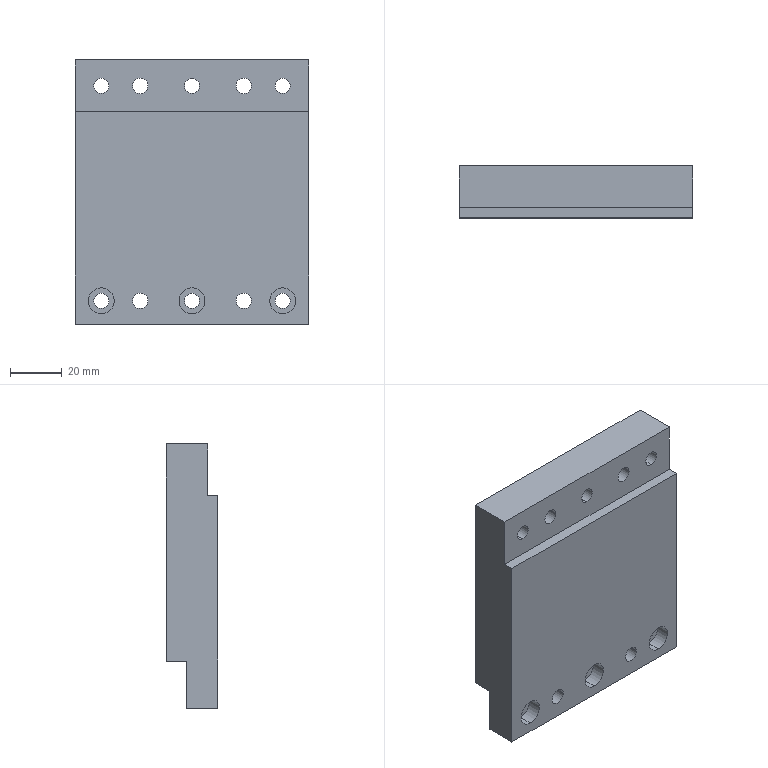Part | NX | features BREP 1 | 1 solid | 48 faces | box 90 x 20 x 102 mm | volume 157949 mm3 | cylinder 32 | plane 16 | commonest cylinder face diameters 5.8 x12 10 x12 6 x8
STEP:
#1=CARTESIAN_POINT('',(35.,20.,36.));
#2=VERTEX_POINT('',#1);
#3=CARTESIAN_POINT('',(35.,14.6,36.));
#4=VERTEX_POINT('',#3);
#5=CARTESIAN_POINT('',(35.,20.,36.));
#6=DIRECTION('',(0.,-1.,0.));
#7=VECTOR('',#6,1000.);
#8=LINE('',#5,#7);
#9=EDGE_CURVE('',#2,#4,#8,.T.);
#10=ORIENTED_EDGE('',*,*,#9,.F.);
#11=CARTESIAN_POINT('',(35.,20.,46.));
#12=VERTEX_POINT('',#11);
#13=CARTESIAN_POINT('',(35.,20.,41.));
#14=DIRECTION('',(0.,-1.,0.));
#15=DIRECTION('',(0.,0.,1.));
#16=AXIS2_PLACEMENT_3D('',#13,#14,#15);
#17=CIRCLE('',#16,5.);
#18=EDGE_CURVE('',#12,#2,#17,.T.);
#19=ORIENTED_EDGE('',*,*,#18,.F.);
#20=CARTESIAN_POINT('',(35.,14.6,46.));
#21=VERTEX_POINT('',#20);
#22=CARTESIAN_POINT('',(35.,20.,46.));
#23=DIRECTION('',(0.,-1.,0.));
#24=VECTOR('',#23,1000.);
#25=LINE('',#22,#24);
#26=EDGE_CURVE('',#12,#21,#25,.T.);
#27=ORIENTED_EDGE('',*,*,#26,.T.);
#28=CARTESIAN_POINT('',(35.,14.6,41.));
#29=DIRECTION('',(0.,1.,0.));
#30=DIRECTION('',(0.,0.,-1.));
#31=AXIS2_PLACEMENT_3D('',#28,#29,#30);
#32=CIRCLE('',#31,5.);
#33=EDGE_CURVE('',#4,#21,#32,.T.);
#34=ORIENTED_EDGE('',*,*,#33,.F.);
#35=EDGE_LOOP('',(#10,#19,#27,#34));
#36=FACE_BOUND('',#35,.T.);
#37=CARTESIAN_POINT('',(35.,20.,41.));
#38=DIRECTION('',(0.,1.,0.));
#39=DIRECTION('',(0.,0.,1.));
#40=AXIS2_PLACEMENT_3D('',#37,#38,#39);
#41=CYLINDRICAL_SURFACE('',#40,5.);
#42=ADVANCED_FACE('',(#36),#41,.F.);
#43=ORIENTED_EDGE('',*,*,#33,.T.);
#44=CARTESIAN_POINT('',(35.,14.6,41.));
#45=DIRECTION('',(0.,1.,0.));
#46=DIRECTION('',(0.,0.,1.));
#47=AXIS2_PLACEMENT_3D('',#44,#45,#46);
#48=CIRCLE('',#47,5.);
#49=EDGE_CURVE('',#21,#4,#48,.T.);
#50=ORIENTED_EDGE('',*,*,#49,.T.);
#51=EDGE_LOOP('',(#43,#50));
#52=FACE_BOUND('',#51,.T.);
#53=CARTESIAN_POINT('',(35.,14.6,43.9));
#54=VERTEX_POINT('',#53);
#55=CARTESIAN_POINT('',(35.,14.6,38.1));
#56=VERTEX_POINT('',#55);
#57=CARTESIAN_POINT('',(35.,14.6,41.));
#58=DIRECTION('',(0.,-1.,0.));
#59=DIRECTION('',(0.,0.,1.));
#60=AXIS2_PLACEMENT_3D('',#57,#58,#59);
#61=CIRCLE('',#60,2.9);
#62=EDGE_CURVE('',#54,#56,#61,.T.);
#63=ORIENTED_EDGE('',*,*,#62,.T.);
#64=CARTESIAN_POINT('',(35.,14.6,41.));
#65=DIRECTION('',(0.,-1.,0.));
#66=DIRECTION('',(0.,0.,-1.));
#67=AXIS2_PLACEMENT_3D('',#64,#65,#66);
#68=CIRCLE('',#67,2.9);
#69=EDGE_CURVE('',#56,#54,#68,.T.);
#70=ORIENTED_EDGE('',*,*,#69,.T.);
#71=EDGE_LOOP('',(#63,#70));
#72=FACE_BOUND('',#71,.T.);
#73=CARTESIAN_POINT('',(37.9,14.6,41.));
#74=DIRECTION('',(0.,-1.,0.));
#75=DIRECTION('',(0.,0.,-1.));
#76=AXIS2_PLACEMENT_3D('',#73,#74,#75);
#77=PLANE('',#76);
#78=ADVANCED_FACE('',(#52,#72),#77,.F.);
#79=ORIENTED_EDGE('',*,*,#49,.F.);
#80=ORIENTED_EDGE('',*,*,#26,.F.);
#81=CARTESIAN_POINT('',(35.,20.,41.));
#82=DIRECTION('',(0.,-1.,0.));
#83=DIRECTION('',(0.,0.,-1.));
#84=AXIS2_PLACEMENT_3D('',#81,#82,#83);
#85=CIRCLE('',#84,5.);
#86=EDGE_CURVE('',#2,#12,#85,.T.);
#87=ORIENTED_EDGE('',*,*,#86,.F.);
#88=ORIENTED_EDGE('',*,*,#9,.T.);
#89=EDGE_LOOP('',(#79,#80,#87,#88));
#90=FACE_BOUND('',#89,.T.);
#91=CARTESIAN_POINT('',(35.,20.,41.));
#92=DIRECTION('',(0.,1.,0.));
#93=DIRECTION('',(0.,0.,1.));
#94=AXIS2_PLACEMENT_3D('',#91,#92,#93);
#95=CYLINDRICAL_SURFACE('',#94,5.);
#96=ADVANCED_FACE('',(#90),#95,.F.);
#97=CARTESIAN_POINT('',(-45.,20.,51.));
#98=VERTEX_POINT('',#97);
#99=CARTESIAN_POINT('',(-45.,20.,-33.));
#100=VERTEX_POINT('',#99);
#101=CARTESIAN_POINT('',(-45.,20.,51.));
#102=DIRECTION('',(0.,0.,-1.));
#103=VECTOR('',#102,1000.);
#104=LINE('',#101,#103);
#105=EDGE_CURVE('',#98,#100,#104,.T.);
#106=ORIENTED_EDGE('',*,*,#105,.F.);
#107=CARTESIAN_POINT('',(45.,20.,51.));
#108=VERTEX_POINT('',#107);
#109=CARTESIAN_POINT('',(45.,20.,51.));
#110=DIRECTION('',(-1.,0.,0.));
#111=VECTOR('',#110,1000.);
#112=LINE('',#109,#111);
#113=EDGE_CURVE('',#108,#98,#112,.T.);
#114=ORIENTED_EDGE('',*,*,#113,.F.);
#115=CARTESIAN_POINT('',(45.,20.,-33.));
#116=VERTEX_POINT('',#115);
#117=CARTESIAN_POINT('',(45.,20.,-33.));
#118=DIRECTION('',(0.,0.,1.));
#119=VECTOR('',#118,1000.);
#120=LINE('',#117,#119);
#121=EDGE_CURVE('',#116,#108,#120,.T.);
#122=ORIENTED_EDGE('',*,*,#121,.F.);
#123=CARTESIAN_POINT('',(45.,20.,-33.));
#124=DIRECTION('',(-1.,0.,0.));
#125=VECTOR('',#124,1000.);
#126=LINE('',#123,#125);
#127=EDGE_CURVE('',#116,#100,#126,.T.);
#128=ORIENTED_EDGE('',*,*,#127,.T.);
#129=EDGE_LOOP('',(#106,#114,#122,#128));
#130=FACE_BOUND('',#129,.T.);
#131=ORIENTED_EDGE('',*,*,#18,.T.);
#132=ORIENTED_EDGE('',*,*,#86,.T.);
#133=EDGE_LOOP('',(#131,#132));
#134=FACE_BOUND('',#133,.T.);
#135=CARTESIAN_POINT('',(0.,20.,46.));
#136=VERTEX_POINT('',#135);
#137=CARTESIAN_POINT('',(0.,20.,36.));
#138=VERTEX_POINT('',#137);
#139=CARTESIAN_POINT('',(0.,20.,41.));
#140=DIRECTION('',(0.,-1.,0.));
#141=DIRECTION('',(0.,0.,1.));
#142=AXIS2_PLACEMENT_3D('',#139,#140,#141);
#143=CIRCLE('',#142,5.);
#144=EDGE_CURVE('',#136,#138,#143,.T.);
#145=ORIENTED_EDGE('',*,*,#144,.T.);
#146=CARTESIAN_POINT('',(0.,20.,41.));
#147=DIRECTION('',(0.,-1.,0.));
#148=DIRECTION('',(0.,0.,-1.));
#149=AXIS2_PLACEMENT_3D('',#146,#147,#148);
#150=CIRCLE('',#149,5.);
#151=EDGE_CURVE('',#138,#136,#150,.T.);
#152=ORIENTED_EDGE('',*,*,#151,.T.);
#153=EDGE_LOOP('',(#145,#152));
#154=FACE_BOUND('',#153,.T.);
#155=CARTESIAN_POINT('',(-35.,20.,46.));
#156=VERTEX_POINT('',#155);
#157=CARTESIAN_POINT('',(-35.,20.,36.));
#158=VERTEX_POINT('',#157);
#159=CARTESIAN_POINT('',(-35.,20.,41.));
#160=DIRECTION('',(0.,-1.,0.));
#161=DIRECTION('',(0.,0.,1.));
#162=AXIS2_PLACEMENT_3D('',#159,#160,#161);
#163=CIRCLE('',#162,5.);
#164=EDGE_CURVE('',#156,#158,#163,.T.);
#165=ORIENTED_EDGE('',*,*,#164,.T.);
#166=CARTESIAN_POINT('',(-35.,20.,41.));
#167=DIRECTION('',(0.,-1.,0.));
#168=DIRECTION('',(0.,0.,-1.));
#169=AXIS2_PLACEMENT_3D('',#166,#167,#168);
#170=CIRCLE('',#169,5.);
#171=EDGE_CURVE('',#158,#156,#170,.T.);
#172=ORIENTED_EDGE('',*,*,#171,.T.);
#173=EDGE_LOOP('',(#165,#172));
#174=FACE_BOUND('',#173,.T.);
#175=CARTESIAN_POINT('',(17.,20.,41.));
#176=VERTEX_POINT('',#175);
#177=CARTESIAN_POINT('',(23.,20.,41.));
#178=VERTEX_POINT('',#177);
#179=CARTESIAN_POINT('',(20.,20.,41.));
#180=DIRECTION('',(0.,-1.,0.));
#181=DIRECTION('',(-1.,0.,0.));
#182=AXIS2_PLACEMENT_3D('',#179,#180,#181);
#183=CIRCLE('',#182,3.);
#184=EDGE_CURVE('',#176,#178,#183,.T.);
#185=ORIENTED_EDGE('',*,*,#184,.T.);
#186=CARTESIAN_POINT('',(20.,20.,41.));
#187=DIRECTION('',(0.,-1.,0.));
#188=DIRECTION('',(1.,0.,0.));
#189=AXIS2_PLACEMENT_3D('',#186,#187,#188);
#190=CIRCLE('',#189,3.);
#191=EDGE_CURVE('',#178,#176,#190,.T.);
#192=ORIENTED_EDGE('',*,*,#191,.T.);
#193=EDGE_LOOP('',(#185,#192));
#194=FACE_BOUND('',#193,.T.);
#195=CARTESIAN_POINT('',(-23.,20.,41.));
#196=VERTEX_POINT('',#195);
#197=CARTESIAN_POINT('',(-17.,20.,41.));
#198=VERTEX_POINT('',#197);
#199=CARTESIAN_POINT('',(-20.,20.,41.));
#200=DIRECTION('',(0.,-1.,0.));
#201=DIRECTION('',(-1.,0.,0.));
#202=AXIS2_PLACEMENT_3D('',#199,#200,#201);
#203=CIRCLE('',#202,3.);
#204=EDGE_CURVE('',#196,#198,#203,.T.);
#205=ORIENTED_EDGE('',*,*,#204,.T.);
#206=CARTESIAN_POINT('',(-20.,20.,41.));
#207=DIRECTION('',(0.,-1.,0.));
#208=DIRECTION('',(1.,0.,0.));
#209=AXIS2_PLACEMENT_3D('',#206,#207,#208);
#210=CIRCLE('',#209,3.);
#211=EDGE_CURVE('',#198,#196,#210,.T.);
#212=ORIENTED_EDGE('',*,*,#211,.T.);
#213=EDGE_LOOP('',(#205,#212));
#214=FACE_BOUND('',#213,.T.);
#215=CARTESIAN_POINT('',(-45.,20.,51.));
#216=DIRECTION('',(0.,1.,0.));
#217=DIRECTION('',(1.,0.,0.));
#218=AXIS2_PLACEMENT_3D('',#215,#216,#217);
#219=PLANE('',#218);
#220=ADVANCED_FACE('',(#130,#134,#154,#174,#194,#214),#219,.T.);
#221=CARTESIAN_POINT('',(45.,12.,-33.));
#222=VERTEX_POINT('',#221);
#223=CARTESIAN_POINT('',(-45.,12.,-33.));
#224=VERTEX_POINT('',#223);
#225=CARTESIAN_POINT('',(45.,12.,-33.));
#226=DIRECTION('',(-1.,0.,0.));
#227=VECTOR('',#226,1000.);
#228=LINE('',#225,#227);
#229=EDGE_CURVE('',#222,#224,#228,.T.);
#230=ORIENTED_EDGE('',*,*,#229,.T.);
#231=CARTESIAN_POINT('',(-45.,12.,-33.));
#232=DIRECTION('',(0.,1.,0.));
#233=VECTOR('',#232,1000.);
#234=LINE('',#231,#233);
#235=EDGE_CURVE('',#224,#100,#234,.T.);
#236=ORIENTED_EDGE('',*,*,#235,.T.);
#237=ORIENTED_EDGE('',*,*,#127,.F.);
#238=CARTESIAN_POINT('',(45.,12.,-33.));
#239=DIRECTION('',(0.,1.,0.));
#240=VECTOR('',#239,1000.);
#241=LINE('',#238,#240);
#242=EDGE_CURVE('',#222,#116,#241,.T.);
#243=ORIENTED_EDGE('',*,*,#242,.F.);
#244=EDGE_LOOP('',(#230,#236,#237,#243));
#245=FACE_BOUND('',#244,.T.);
#246=CARTESIAN_POINT('',(-45.,20.,-33.));
#247=DIRECTION('',(0.,0.,1.));
#248=DIRECTION('',(1.,0.,0.));
#249=AXIS2_PLACEMENT_3D('',#246,#247,#248);
#250=PLANE('',#249);
#251=ADVANCED_FACE('',(#245),#250,.F.);
#252=CARTESIAN_POINT('',(45.,0.,31.));
#253=VERTEX_POINT('',#252);
#254=CARTESIAN_POINT('',(45.,4.,31.));
#255=VERTEX_POINT('',#254);
#256=CARTESIAN_POINT('',(45.,0.,31.));
#257=DIRECTION('',(0.,1.,0.));
#258=VECTOR('',#257,1000.);
#259=LINE('',#256,#258);
#260=EDGE_CURVE('',#253,#255,#259,.T.);
#261=ORIENTED_EDGE('',*,*,#260,.F.);
#262=CARTESIAN_POINT('',(45.,0.,-51.));
#263=VERTEX_POINT('',#262);
#264=CARTESIAN_POINT('',(45.,0.,-51.));
#265=DIRECTION('',(0.,0.,1.));
#266=VECTOR('',#265,1000.);
#267=LINE('',#264,#266);
#268=EDGE_CURVE('',#263,#253,#267,.T.);
#269=ORIENTED_EDGE('',*,*,#268,.F.);
#270=CARTESIAN_POINT('',(45.,12.,-51.));
#271=VERTEX_POINT('',#270);
#272=CARTESIAN_POINT('',(45.,0.,-51.));
#273=DIRECTION('',(0.,1.,0.));
#274=VECTOR('',#273,1000.);
#275=LINE('',#272,#274);
#276=EDGE_CURVE('',#263,#271,#275,.T.);
#277=ORIENTED_EDGE('',*,*,#276,.T.);
#278=CARTESIAN_POINT('',(45.,12.,-51.));
#279=DIRECTION('',(0.,0.,1.));
#280=VECTOR('',#279,1000.);
#281=LINE('',#278,#280);
#282=EDGE_CURVE('',#271,#222,#281,.T.);
#283=ORIENTED_EDGE('',*,*,#282,.T.);
#284=ORIENTED_EDGE('',*,*,#242,.T.);
#285=ORIENTED_EDGE('',*,*,#121,.T.);
#286=CARTESIAN_POINT('',(45.,4.,51.));
#287=VERTEX_POINT('',#286);
#288=CARTESIAN_POINT('',(45.,4.,51.));
#289=DIRECTION('',(0.,1.,0.));
#290=VECTOR('',#289,1000.);
#291=LINE('',#288,#290);
#292=EDGE_CURVE('',#287,#108,#291,.T.);
#293=ORIENTED_EDGE('',*,*,#292,.F.);
#294=CARTESIAN_POINT('',(45.,4.,51.));
#295=DIRECTION('',(0.,0.,-1.));
#296=VECTOR('',#295,1000.);
#297=LINE('',#294,#296);
#298=EDGE_CURVE('',#287,#255,#297,.T.);
#299=ORIENTED_EDGE('',*,*,#298,.T.);
#300=EDGE_LOOP('',(#261,#269,#277,#283,#284,#285,#293,#299));
#301=FACE_BOUND('',#300,.T.);
#302=CARTESIAN_POINT('',(45.,20.,-51.));
#303=DIRECTION('',(-1.,0.,0.));
#304=DIRECTION('',(0.,0.,1.));
#305=AXIS2_PLACEMENT_3D('',#302,#303,#304);
#306=PLANE('',#305);
#307=ADVANCED_FACE('',(#301),#306,.F.);
#308=CARTESIAN_POINT('',(-45.,4.,31.));
#309=VERTEX_POINT('',#308);
#310=CARTESIAN_POINT('',(45.,4.,31.));
#311=DIRECTION('',(-1.,0.,0.));
#312=VECTOR('',#311,1000.);
#313=LINE('',#310,#312);
#314=EDGE_CURVE('',#255,#309,#313,.T.);
#315=ORIENTED_EDGE('',*,*,#314,.F.);
#316=ORIENTED_EDGE('',*,*,#298,.F.);
#317=CARTESIAN_POINT('',(-45.,4.,51.));
#318=VERTEX_POINT('',#317);
#319=CARTESIAN_POINT('',(-45.,4.,51.));
#320=DIRECTION('',(1.,0.,0.));
#321=VECTOR('',#320,1000.);
#322=LINE('',#319,#321);
#323=EDGE_CURVE('',#318,#287,#322,.T.);
#324=ORIENTED_EDGE('',*,*,#323,.F.);
#325=CARTESIAN_POINT('',(-45.,4.,31.));
#326=DIRECTION('',(0.,0.,1.));
#327=VECTOR('',#326,1000.);
#328=LINE('',#325,#327);
#329=EDGE_CURVE('',#309,#318,#328,.T.);
#330=ORIENTED_EDGE('',*,*,#329,.F.);
#331=EDGE_LOOP('',(#315,#316,#324,#330));
#332=FACE_BOUND('',#331,.T.);
#333=CARTESIAN_POINT('',(0.,4.,38.1));
#334=VERTEX_POINT('',#333);
#335=CARTESIAN_POINT('',(0.,4.,43.9));
#336=VERTEX_POINT('',#335);
#337=CARTESIAN_POINT('',(0.,4.,41.));
#338=DIRECTION('',(0.,1.,0.));
#339=DIRECTION('',(0.,0.,-1.));
#340=AXIS2_PLACEMENT_3D('',#337,#338,#339);
#341=CIRCLE('',#340,2.9);
#342=EDGE_CURVE('',#334,#336,#341,.T.);
#343=ORIENTED_EDGE('',*,*,#342,.T.);
#344=CARTESIAN_POINT('',(0.,4.,41.));
#345=DIRECTION('',(0.,1.,0.));
#346=DIRECTION('',(0.,0.,1.));
#347=AXIS2_PLACEMENT_3D('',#344,#345,#346);
#348=CIRCLE('',#347,2.9);
#349=EDGE_CURVE('',#336,#334,#348,.T.);
#350=ORIENTED_EDGE('',*,*,#349,.T.);
#351=EDGE_LOOP('',(#343,#350));
#352=FACE_BOUND('',#351,.T.);
#353=CARTESIAN_POINT('',(35.,4.,38.1));
#354=VERTEX_POINT('',#353);
#355=CARTESIAN_POINT('',(35.,4.,43.9));
#356=VERTEX_POINT('',#355);
#357=CARTESIAN_POINT('',(35.,4.,41.));
#358=DIRECTION('',(0.,1.,0.));
#359=DIRECTION('',(0.,0.,-1.));
#360=AXIS2_PLACEMENT_3D('',#357,#358,#359);
#361=CIRCLE('',#360,2.9);
#362=EDGE_CURVE('',#354,#356,#361,.T.);
#363=ORIENTED_EDGE('',*,*,#362,.T.);
#364=CARTESIAN_POINT('',(35.,4.,41.));
#365=DIRECTION('',(0.,1.,0.));
#366=DIRECTION('',(0.,0.,1.));
#367=AXIS2_PLACEMENT_3D('',#364,#365,#366);
#368=CIRCLE('',#367,2.9);
#369=EDGE_CURVE('',#356,#354,#368,.T.);
#370=ORIENTED_EDGE('',*,*,#369,.T.);
#371=EDGE_LOOP('',(#363,#370));
#372=FACE_BOUND('',#371,.T.);
#373=CARTESIAN_POINT('',(-35.,4.,38.1));
#374=VERTEX_POINT('',#373);
#375=CARTESIAN_POINT('',(-35.,4.,43.9));
#376=VERTEX_POINT('',#375);
#377=CARTESIAN_POINT('',(-35.,4.,41.));
#378=DIRECTION('',(0.,1.,0.));
#379=DIRECTION('',(0.,0.,-1.));
#380=AXIS2_PLACEMENT_3D('',#377,#378,#379);
#381=CIRCLE('',#380,2.9);
#382=EDGE_CURVE('',#374,#376,#381,.T.);
#383=ORIENTED_EDGE('',*,*,#382,.T.);
#384=CARTESIAN_POINT('',(-35.,4.,41.));
#385=DIRECTION('',(0.,1.,0.));
#386=DIRECTION('',(0.,0.,1.));
#387=AXIS2_PLACEMENT_3D('',#384,#385,#386);
#388=CIRCLE('',#387,2.9);
#389=EDGE_CURVE('',#376,#374,#388,.T.);
#390=ORIENTED_EDGE('',*,*,#389,.T.);
#391=EDGE_LOOP('',(#383,#390));
#392=FACE_BOUND('',#391,.T.);
#393=CARTESIAN_POINT('',(17.,4.,41.));
#394=VERTEX_POINT('',#393);
#395=CARTESIAN_POINT('',(23.,4.,41.));
#396=VERTEX_POINT('',#395);
#397=CARTESIAN_POINT('',(20.,4.,41.));
#398=DIRECTION('',(0.,-1.,0.));
#399=DIRECTION('',(-1.,0.,0.));
#400=AXIS2_PLACEMENT_3D('',#397,#398,#399);
#401=CIRCLE('',#400,3.);
#402=EDGE_CURVE('',#394,#396,#401,.T.);
#403=ORIENTED_EDGE('',*,*,#402,.F.);
#404=CARTESIAN_POINT('',(20.,4.,41.));
#405=DIRECTION('',(0.,-1.,0.));
#406=DIRECTION('',(1.,0.,0.));
#407=AXIS2_PLACEMENT_3D('',#404,#405,#406);
#408=CIRCLE('',#407,3.);
#409=EDGE_CURVE('',#396,#394,#408,.T.);
#410=ORIENTED_EDGE('',*,*,#409,.F.);
#411=EDGE_LOOP('',(#403,#410));
#412=FACE_BOUND('',#411,.T.);
#413=CARTESIAN_POINT('',(-23.,4.,41.));
#414=VERTEX_POINT('',#413);
#415=CARTESIAN_POINT('',(-17.,4.,41.));
#416=VERTEX_POINT('',#415);
#417=CARTESIAN_POINT('',(-20.,4.,41.));
#418=DIRECTION('',(0.,-1.,0.));
#419=DIRECTION('',(-1.,0.,0.));
#420=AXIS2_PLACEMENT_3D('',#417,#418,#419);
#421=CIRCLE('',#420,3.);
#422=EDGE_CURVE('',#414,#416,#421,.T.);
#423=ORIENTED_EDGE('',*,*,#422,.F.);
#424=CARTESIAN_POINT('',(-20.,4.,41.));
#425=DIRECTION('',(0.,-1.,0.));
#426=DIRECTION('',(1.,0.,0.));
#427=AXIS2_PLACEMENT_3D('',#424,#425,#426);
#428=CIRCLE('',#427,3.);
#429=EDGE_CURVE('',#416,#414,#428,.T.);
#430=ORIENTED_EDGE('',*,*,#429,.F.);
#431=EDGE_LOOP('',(#423,#430));
#432=FACE_BOUND('',#431,.T.);
#433=CARTESIAN_POINT('',(-45.,4.,31.));
#434=DIRECTION('',(0.,-1.,0.));
#435=DIRECTION('',(0.,0.,-1.));
#436=AXIS2_PLACEMENT_3D('',#433,#434,#435);
#437=PLANE('',#436);
#438=ADVANCED_FACE('',(#332,#352,#372,#392,#412,#432),#437,.T.);
#439=CARTESIAN_POINT('',(-45.,0.,31.));
#440=VERTEX_POINT('',#439);
#441=CARTESIAN_POINT('',(-45.,0.,31.));
#442=DIRECTION('',(0.,1.,0.));
#443=VECTOR('',#442,1000.);
#444=LINE('',#441,#443);
#445=EDGE_CURVE('',#440,#309,#444,.T.);
#446=ORIENTED_EDGE('',*,*,#445,.T.);
#447=ORIENTED_EDGE('',*,*,#329,.T.);
#448=CARTESIAN_POINT('',(-45.,4.,51.));
#449=DIRECTION('',(0.,1.,0.));
#450=VECTOR('',#449,1000.);
#451=LINE('',#448,#450);
#452=EDGE_CURVE('',#318,#98,#451,.T.);
#453=ORIENTED_EDGE('',*,*,#452,.T.);
#454=ORIENTED_EDGE('',*,*,#105,.T.);
#455=ORIENTED_EDGE('',*,*,#235,.F.);
#456=CARTESIAN_POINT('',(-45.,12.,-51.));
#457=VERTEX_POINT('',#456);
#458=CARTESIAN_POINT('',(-45.,12.,-51.));
#459=DIRECTION('',(0.,0.,1.));
#460=VECTOR('',#459,1000.);
#461=LINE('',#458,#460);
#462=EDGE_CURVE('',#457,#224,#461,.T.);
#463=ORIENTED_EDGE('',*,*,#462,.F.);
#464=CARTESIAN_POINT('',(-45.,0.,-51.));
#465=VERTEX_POINT('',#464);
#466=CARTESIAN_POINT('',(-45.,0.,-51.));
#467=DIRECTION('',(0.,1.,0.));
#468=VECTOR('',#467,1000.);
#469=LINE('',#466,#468);
#470=EDGE_CURVE('',#465,#457,#469,.T.);
#471=ORIENTED_EDGE('',*,*,#470,.F.);
#472=CARTESIAN_POINT('',(-45.,0.,31.));
#473=DIRECTION('',(0.,0.,-1.));
#474=VECTOR('',#473,1000.);
#475=LINE('',#472,#474);
#476=EDGE_CURVE('',#440,#465,#475,.T.);
#477=ORIENTED_EDGE('',*,*,#476,.F.);
#478=EDGE_LOOP('',(#446,#447,#453,#454,#455,#463,#471,#477));
#479=FACE_BOUND('',#478,.T.);
#480=CARTESIAN_POINT('',(-45.,20.,-51.));
#481=DIRECTION('',(1.,0.,0.));
#482=DIRECTION('',(0.,1.,0.));
#483=AXIS2_PLACEMENT_3D('',#480,#481,#482);
#484=PLANE('',#483);
#485=ADVANCED_FACE('',(#479),#484,.F.);
#486=CARTESIAN_POINT('',(45.,0.,31.));
#487=DIRECTION('',(-1.,0.,0.));
#488=VECTOR('',#487,1000.);
#489=LINE('',#486,#488);
#490=EDGE_CURVE('',#253,#440,#489,.T.);
#491=ORIENTED_EDGE('',*,*,#490,.T.);
#492=ORIENTED_EDGE('',*,*,#476,.T.);
#493=CARTESIAN_POINT('',(-45.,0.,-51.));
#494=DIRECTION('',(1.,0.,0.));
#495=VECTOR('',#494,1000.);
#496=LINE('',#493,#495);
#497=EDGE_CURVE('',#465,#263,#496,.T.);
#498=ORIENTED_EDGE('',*,*,#497,.T.);
#499=ORIENTED_EDGE('',*,*,#268,.T.);
#500=EDGE_LOOP('',(#491,#492,#498,#499));
#501=FACE_BOUND('',#500,.T.);
#502=CARTESIAN_POINT('',(0.,0.,-47.));
#503=VERTEX_POINT('',#502);
#504=CARTESIAN_POINT('',(0.,0.,-37.));
#505=VERTEX_POINT('',#504);
#506=CARTESIAN_POINT('',(0.,0.,-42.));
#507=DIRECTION('',(0.,1.,0.));
#508=DIRECTION('',(0.,0.,-1.));
#509=AXIS2_PLACEMENT_3D('',#506,#507,#508);
#510=CIRCLE('',#509,5.);
#511=EDGE_CURVE('',#503,#505,#510,.T.);
#512=ORIENTED_EDGE('',*,*,#511,.T.);
#513=CARTESIAN_POINT('',(0.,0.,-42.));
#514=DIRECTION('',(0.,1.,0.));
#515=DIRECTION('',(0.,0.,1.));
#516=AXIS2_PLACEMENT_3D('',#513,#514,#515);
#517=CIRCLE('',#516,5.);
#518=EDGE_CURVE('',#505,#503,#517,.T.);
#519=ORIENTED_EDGE('',*,*,#518,.T.);
#520=EDGE_LOOP('',(#512,#519));
#521=FACE_BOUND('',#520,.T.);
#522=CARTESIAN_POINT('',(35.,0.,-47.));
#523=VERTEX_POINT('',#522);
#524=CARTESIAN_POINT('',(35.,0.,-37.));
#525=VERTEX_POINT('',#524);
#526=CARTESIAN_POINT('',(35.,0.,-42.));
#527=DIRECTION('',(0.,1.,0.));
#528=DIRECTION('',(0.,0.,-1.));
#529=AXIS2_PLACEMENT_3D('',#526,#527,#528);
#530=CIRCLE('',#529,5.);
#531=EDGE_CURVE('',#523,#525,#530,.T.);
#532=ORIENTED_EDGE('',*,*,#531,.T.);
#533=CARTESIAN_POINT('',(35.,0.,-42.));
#534=DIRECTION('',(0.,1.,0.));
#535=DIRECTION('',(0.,0.,1.));
#536=AXIS2_PLACEMENT_3D('',#533,#534,#535);
#537=CIRCLE('',#536,5.);
#538=EDGE_CURVE('',#525,#523,#537,.T.);
#539=ORIENTED_EDGE('',*,*,#538,.T.);
#540=EDGE_LOOP('',(#532,#539));
#541=FACE_BOUND('',#540,.T.);
#542=CARTESIAN_POINT('',(-35.,0.,-47.));
#543=VERTEX_POINT('',#542);
#544=CARTESIAN_POINT('',(-35.,0.,-37.));
#545=VERTEX_POINT('',#544);
#546=CARTESIAN_POINT('',(-35.,0.,-42.));
#547=DIRECTION('',(0.,1.,0.));
#548=DIRECTION('',(0.,0.,-1.));
#549=AXIS2_PLACEMENT_3D('',#546,#547,#548);
#550=CIRCLE('',#549,5.);
#551=EDGE_CURVE('',#543,#545,#550,.T.);
#552=ORIENTED_EDGE('',*,*,#551,.T.);
#553=CARTESIAN_POINT('',(-35.,0.,-42.));
#554=DIRECTION('',(0.,1.,0.));
#555=DIRECTION('',(0.,0.,1.));
#556=AXIS2_PLACEMENT_3D('',#553,#554,#555);
#557=CIRCLE('',#556,5.);
#558=EDGE_CURVE('',#545,#543,#557,.T.);
#559=ORIENTED_EDGE('',*,*,#558,.T.);
#560=EDGE_LOOP('',(#552,#559));
#561=FACE_BOUND('',#560,.T.);
#562=CARTESIAN_POINT('',(-17.,0.,-42.));
#563=VERTEX_POINT('',#562);
#564=CARTESIAN_POINT('',(-23.,0.,-42.));
#565=VERTEX_POINT('',#564);
#566=CARTESIAN_POINT('',(-20.,0.,-42.));
#567=DIRECTION('',(0.,1.,0.));
#568=DIRECTION('',(1.,0.,0.));
#569=AXIS2_PLACEMENT_3D('',#566,#567,#568);
#570=CIRCLE('',#569,3.);
#571=EDGE_CURVE('',#563,#565,#570,.T.);
#572=ORIENTED_EDGE('',*,*,#571,.T.);
#573=CARTESIAN_POINT('',(-20.,0.,-42.));
#574=DIRECTION('',(0.,1.,0.));
#575=DIRECTION('',(-1.,0.,0.));
#576=AXIS2_PLACEMENT_3D('',#573,#574,#575);
#577=CIRCLE('',#576,3.);
#578=EDGE_CURVE('',#565,#563,#577,.T.);
#579=ORIENTED_EDGE('',*,*,#578,.T.);
#580=EDGE_LOOP('',(#572,#579));
#581=FACE_BOUND('',#580,.T.);
#582=CARTESIAN_POINT('',(23.,0.,-42.));
#583=VERTEX_POINT('',#582);
#584=CARTESIAN_POINT('',(17.,0.,-42.));
#585=VERTEX_POINT('',#584);
#586=CARTESIAN_POINT('',(20.,0.,-42.));
#587=DIRECTION('',(0.,1.,0.));
#588=DIRECTION('',(1.,0.,0.));
#589=AXIS2_PLACEMENT_3D('',#586,#587,#588);
#590=CIRCLE('',#589,3.);
#591=EDGE_CURVE('',#583,#585,#590,.T.);
#592=ORIENTED_EDGE('',*,*,#591,.T.);
#593=CARTESIAN_POINT('',(20.,0.,-42.));
#594=DIRECTION('',(0.,1.,0.));
#595=DIRECTION('',(-1.,0.,0.));
#596=AXIS2_PLACEMENT_3D('',#593,#594,#595);
#597=CIRCLE('',#596,3.);
#598=EDGE_CURVE('',#585,#583,#597,.T.);
#599=ORIENTED_EDGE('',*,*,#598,.T.);
#600=EDGE_LOOP('',(#592,#599));
#601=FACE_BOUND('',#600,.T.);
#602=CARTESIAN_POINT('',(-45.,0.,51.));
#603=DIRECTION('',(0.,1.,0.));
#604=DIRECTION('',(1.,0.,0.));
#605=AXIS2_PLACEMENT_3D('',#602,#603,#604);
#606=PLANE('',#605);
#607=ADVANCED_FACE('',(#501,#521,#541,#561,#581,#601),#606,.F.);
#608=CARTESIAN_POINT('',(45.,12.,-51.));
#609=DIRECTION('',(-1.,0.,0.));
#610=VECTOR('',#609,1000.);
#611=LINE('',#608,#610);
#612=EDGE_CURVE('',#271,#457,#611,.T.);
#613=ORIENTED_EDGE('',*,*,#612,.F.);
#614=ORIENTED_EDGE('',*,*,#276,.F.);
#615=ORIENTED_EDGE('',*,*,#497,.F.);
#616=ORIENTED_EDGE('',*,*,#470,.T.);
#617=EDGE_LOOP('',(#613,#614,#615,#616));
#618=FACE_BOUND('',#617,.T.);
#619=CARTESIAN_POINT('',(-45.,20.,-51.));
#620=DIRECTION('',(0.,0.,1.));
#621=DIRECTION('',(1.,0.,0.));
#622=AXIS2_PLACEMENT_3D('',#619,#620,#621);
#623=PLANE('',#622);
#624=ADVANCED_FACE('',(#618),#623,.F.);
#625=ORIENTED_EDGE('',*,*,#612,.T.);
#626=ORIENTED_EDGE('',*,*,#462,.T.);
#627=ORIENTED_EDGE('',*,*,#229,.F.);
#628=ORIENTED_EDGE('',*,*,#282,.F.);
#629=EDGE_LOOP('',(#625,#626,#627,#628));
#630=FACE_BOUND('',#629,.T.);
#631=CARTESIAN_POINT('',(0.,12.,-39.1));
#632=VERTEX_POINT('',#631);
#633=CARTESIAN_POINT('',(0.,12.,-44.9));
#634=VERTEX_POINT('',#633);
#635=CARTESIAN_POINT('',(0.,12.,-42.));
#636=DIRECTION('',(0.,-1.,0.));
#637=DIRECTION('',(0.,0.,1.));
#638=AXIS2_PLACEMENT_3D('',#635,#636,#637);
#639=CIRCLE('',#638,2.9);
#640=EDGE_CURVE('',#632,#634,#639,.T.);
#641=ORIENTED_EDGE('',*,*,#640,.T.);
#642=CARTESIAN_POINT('',(0.,12.,-42.));
#643=DIRECTION('',(0.,-1.,0.));
#644=DIRECTION('',(0.,0.,-1.));
#645=AXIS2_PLACEMENT_3D('',#642,#643,#644);
#646=CIRCLE('',#645,2.9);
#647=EDGE_CURVE('',#634,#632,#646,.T.);
#648=ORIENTED_EDGE('',*,*,#647,.T.);
#649=EDGE_LOOP('',(#641,#648));
#650=FACE_BOUND('',#649,.T.);
#651=CARTESIAN_POINT('',(35.,12.,-39.1));
#652=VERTEX_POINT('',#651);
#653=CARTESIAN_POINT('',(35.,12.,-44.9));
#654=VERTEX_POINT('',#653);
#655=CARTESIAN_POINT('',(35.,12.,-42.));
#656=DIRECTION('',(0.,-1.,0.));
#657=DIRECTION('',(0.,0.,1.));
#658=AXIS2_PLACEMENT_3D('',#655,#656,#657);
#659=CIRCLE('',#658,2.9);
#660=EDGE_CURVE('',#652,#654,#659,.T.);
#661=ORIENTED_EDGE('',*,*,#660,.T.);
#662=CARTESIAN_POINT('',(35.,12.,-42.));
#663=DIRECTION('',(0.,-1.,0.));
#664=DIRECTION('',(0.,0.,-1.));
#665=AXIS2_PLACEMENT_3D('',#662,#663,#664);
#666=CIRCLE('',#665,2.9);
#667=EDGE_CURVE('',#654,#652,#666,.T.);
#668=ORIENTED_EDGE('',*,*,#667,.T.);
#669=EDGE_LOOP('',(#661,#668));
#670=FACE_BOUND('',#669,.T.);
#671=CARTESIAN_POINT('',(-35.,12.,-39.1));
#672=VERTEX_POINT('',#671);
#673=CARTESIAN_POINT('',(-35.,12.,-44.9));
#674=VERTEX_POINT('',#673);
#675=CARTESIAN_POINT('',(-35.,12.,-42.));
#676=DIRECTION('',(0.,-1.,0.));
#677=DIRECTION('',(0.,0.,1.));
#678=AXIS2_PLACEMENT_3D('',#675,#676,#677);
#679=CIRCLE('',#678,2.9);
#680=EDGE_CURVE('',#672,#674,#679,.T.);
#681=ORIENTED_EDGE('',*,*,#680,.T.);
#682=CARTESIAN_POINT('',(-35.,12.,-42.));
#683=DIRECTION('',(0.,-1.,0.));
#684=DIRECTION('',(0.,0.,-1.));
#685=AXIS2_PLACEMENT_3D('',#682,#683,#684);
#686=CIRCLE('',#685,2.9);
#687=EDGE_CURVE('',#674,#672,#686,.T.);
#688=ORIENTED_EDGE('',*,*,#687,.T.);
#689=EDGE_LOOP('',(#681,#688));
#690=FACE_BOUND('',#689,.T.);
#691=CARTESIAN_POINT('',(-17.,12.,-42.));
#692=VERTEX_POINT('',#691);
#693=CARTESIAN_POINT('',(-23.,12.,-42.));
#694=VERTEX_POINT('',#693);
#695=CARTESIAN_POINT('',(-20.,12.,-42.));
#696=DIRECTION('',(0.,1.,0.));
#697=DIRECTION('',(1.,0.,0.));
#698=AXIS2_PLACEMENT_3D('',#695,#696,#697);
#699=CIRCLE('',#698,3.);
#700=EDGE_CURVE('',#692,#694,#699,.T.);
#701=ORIENTED_EDGE('',*,*,#700,.F.);
#702=CARTESIAN_POINT('',(-20.,12.,-42.));
#703=DIRECTION('',(0.,1.,0.));
#704=DIRECTION('',(-1.,0.,0.));
#705=AXIS2_PLACEMENT_3D('',#702,#703,#704);
#706=CIRCLE('',#705,3.);
#707=EDGE_CURVE('',#694,#692,#706,.T.);
#708=ORIENTED_EDGE('',*,*,#707,.F.);
#709=EDGE_LOOP('',(#701,#708));
#710=FACE_BOUND('',#709,.T.);
#711=CARTESIAN_POINT('',(23.,12.,-42.));
#712=VERTEX_POINT('',#711);
#713=CARTESIAN_POINT('',(17.,12.,-42.));
#714=VERTEX_POINT('',#713);
#715=CARTESIAN_POINT('',(20.,12.,-42.));
#716=DIRECTION('',(0.,1.,0.));
#717=DIRECTION('',(1.,0.,0.));
#718=AXIS2_PLACEMENT_3D('',#715,#716,#717);
#719=CIRCLE('',#718,3.);
#720=EDGE_CURVE('',#712,#714,#719,.T.);
#721=ORIENTED_EDGE('',*,*,#720,.F.);
#722=CARTESIAN_POINT('',(20.,12.,-42.));
#723=DIRECTION('',(0.,1.,0.));
#724=DIRECTION('',(-1.,0.,0.));
#725=AXIS2_PLACEMENT_3D('',#722,#723,#724);
#726=CIRCLE('',#725,3.);
#727=EDGE_CURVE('',#714,#712,#726,.T.);
#728=ORIENTED_EDGE('',*,*,#727,.F.);
#729=EDGE_LOOP('',(#721,#728));
#730=FACE_BOUND('',#729,.T.);
#731=CARTESIAN_POINT('',(-45.,12.,-51.));
#732=DIRECTION('',(0.,-1.,0.));
#733=DIRECTION('',(0.,0.,-1.));
#734=AXIS2_PLACEMENT_3D('',#731,#732,#733);
#735=PLANE('',#734);
#736=ADVANCED_FACE('',(#630,#650,#670,#690,#710,#730),#735,.F.);
#737=ORIENTED_EDGE('',*,*,#647,.F.);
#738=CARTESIAN_POINT('',(0.,5.4,-44.9));
#739=VERTEX_POINT('',#738);
#740=CARTESIAN_POINT('',(0.,5.4,-44.9));
#741=DIRECTION('',(0.,1.,0.));
#742=VECTOR('',#741,1000.);
#743=LINE('',#740,#742);
#744=EDGE_CURVE('',#739,#634,#743,.T.);
#745=ORIENTED_EDGE('',*,*,#744,.F.);
#746=CARTESIAN_POINT('',(0.,5.4,-39.1));
#747=VERTEX_POINT('',#746);
#748=CARTESIAN_POINT('',(0.,5.4,-42.));
#749=DIRECTION('',(0.,1.,0.));
#750=DIRECTION('',(0.,0.,1.));
#751=AXIS2_PLACEMENT_3D('',#748,#749,#750);
#752=CIRCLE('',#751,2.9);
#753=EDGE_CURVE('',#747,#739,#752,.T.);
#754=ORIENTED_EDGE('',*,*,#753,.F.);
#755=CARTESIAN_POINT('',(0.,5.4,-39.1));
#756=DIRECTION('',(0.,1.,0.));
#757=VECTOR('',#756,1000.);
#758=LINE('',#755,#757);
#759=EDGE_CURVE('',#747,#632,#758,.T.);
#760=ORIENTED_EDGE('',*,*,#759,.T.);
#761=EDGE_LOOP('',(#737,#745,#754,#760));
#762=FACE_BOUND('',#761,.T.);
#763=CARTESIAN_POINT('',(0.,0.,-42.));
#764=DIRECTION('',(0.,-1.,0.));
#765=DIRECTION('',(0.,0.,-1.));
#766=AXIS2_PLACEMENT_3D('',#763,#764,#765);
#767=CYLINDRICAL_SURFACE('',#766,2.9);
#768=ADVANCED_FACE('',(#762),#767,.F.);
#769=ORIENTED_EDGE('',*,*,#640,.F.);
#770=ORIENTED_EDGE('',*,*,#759,.F.);
#771=CARTESIAN_POINT('',(0.,5.4,-42.));
#772=DIRECTION('',(0.,1.,0.));
#773=DIRECTION('',(0.,0.,-1.));
#774=AXIS2_PLACEMENT_3D('',#771,#772,#773);
#775=CIRCLE('',#774,2.9);
#776=EDGE_CURVE('',#739,#747,#775,.T.);
#777=ORIENTED_EDGE('',*,*,#776,.F.);
#778=ORIENTED_EDGE('',*,*,#744,.T.);
#779=EDGE_LOOP('',(#769,#770,#777,#778));
#780=FACE_BOUND('',#779,.T.);
#781=CARTESIAN_POINT('',(0.,0.,-42.));
#782=DIRECTION('',(0.,-1.,0.));
#783=DIRECTION('',(0.,0.,-1.));
#784=AXIS2_PLACEMENT_3D('',#781,#782,#783);
#785=CYLINDRICAL_SURFACE('',#784,2.9);
#786=ADVANCED_FACE('',(#780),#785,.F.);
#787=CARTESIAN_POINT('',(0.,5.4,-37.));
#788=VERTEX_POINT('',#787);
#789=CARTESIAN_POINT('',(0.,5.4,-47.));
#790=VERTEX_POINT('',#789);
#791=CARTESIAN_POINT('',(0.,5.4,-42.));
#792=DIRECTION('',(0.,-1.,0.));
#793=DIRECTION('',(0.,0.,1.));
#794=AXIS2_PLACEMENT_3D('',#791,#792,#793);
#795=CIRCLE('',#794,5.);
#796=EDGE_CURVE('',#788,#790,#795,.T.);
#797=ORIENTED_EDGE('',*,*,#796,.T.);
#798=CARTESIAN_POINT('',(0.,5.4,-42.));
#799=DIRECTION('',(0.,-1.,0.));
#800=DIRECTION('',(0.,0.,-1.));
#801=AXIS2_PLACEMENT_3D('',#798,#799,#800);
#802=CIRCLE('',#801,5.);
#803=EDGE_CURVE('',#790,#788,#802,.T.);
#804=ORIENTED_EDGE('',*,*,#803,.T.);
#805=EDGE_LOOP('',(#797,#804));
#806=FACE_BOUND('',#805,.T.);
#807=ORIENTED_EDGE('',*,*,#776,.T.);
#808=ORIENTED_EDGE('',*,*,#753,.T.);
#809=EDGE_LOOP('',(#807,#808));
#810=FACE_BOUND('',#809,.T.);
#811=CARTESIAN_POINT('',(2.9,5.4,-42.));
#812=DIRECTION('',(0.,1.,0.));
#813=DIRECTION('',(1.,0.,0.));
#814=AXIS2_PLACEMENT_3D('',#811,#812,#813);
#815=PLANE('',#814);
#816=ADVANCED_FACE('',(#806,#810),#815,.F.);
#817=ORIENTED_EDGE('',*,*,#803,.F.);
#818=CARTESIAN_POINT('',(0.,0.,-47.));
#819=DIRECTION('',(0.,1.,0.));
#820=VECTOR('',#819,1000.);
#821=LINE('',#818,#820);
#822=EDGE_CURVE('',#503,#790,#821,.T.);
#823=ORIENTED_EDGE('',*,*,#822,.F.);
#824=ORIENTED_EDGE('',*,*,#518,.F.);
#825=CARTESIAN_POINT('',(0.,0.,-37.));
#826=DIRECTION('',(0.,1.,0.));
#827=VECTOR('',#826,1000.);
#828=LINE('',#825,#827);
#829=EDGE_CURVE('',#505,#788,#828,.T.);
#830=ORIENTED_EDGE('',*,*,#829,.T.);
#831=EDGE_LOOP('',(#817,#823,#824,#830));
#832=FACE_BOUND('',#831,.T.);
#833=CARTESIAN_POINT('',(0.,0.,-42.));
#834=DIRECTION('',(0.,-1.,0.));
#835=DIRECTION('',(0.,0.,-1.));
#836=AXIS2_PLACEMENT_3D('',#833,#834,#835);
#837=CYLINDRICAL_SURFACE('',#836,5.);
#838=ADVANCED_FACE('',(#832),#837,.F.);
#839=ORIENTED_EDGE('',*,*,#829,.F.);
#840=ORIENTED_EDGE('',*,*,#511,.F.);
#841=ORIENTED_EDGE('',*,*,#822,.T.);
#842=ORIENTED_EDGE('',*,*,#796,.F.);
#843=EDGE_LOOP('',(#839,#840,#841,#842));
#844=FACE_BOUND('',#843,.T.);
#845=CARTESIAN_POINT('',(0.,0.,-42.));
#846=DIRECTION('',(0.,-1.,0.));
#847=DIRECTION('',(0.,0.,-1.));
#848=AXIS2_PLACEMENT_3D('',#845,#846,#847);
#849=CYLINDRICAL_SURFACE('',#848,5.);
#850=ADVANCED_FACE('',(#844),#849,.F.);
#851=ORIENTED_EDGE('',*,*,#667,.F.);
#852=CARTESIAN_POINT('',(35.,5.4,-44.9));
#853=VERTEX_POINT('',#852);
#854=CARTESIAN_POINT('',(35.,5.4,-44.9));
#855=DIRECTION('',(0.,1.,0.));
#856=VECTOR('',#855,1000.);
#857=LINE('',#854,#856);
#858=EDGE_CURVE('',#853,#654,#857,.T.);
#859=ORIENTED_EDGE('',*,*,#858,.F.);
#860=CARTESIAN_POINT('',(35.,5.4,-39.1));
#861=VERTEX_POINT('',#860);
#862=CARTESIAN_POINT('',(35.,5.4,-42.));
#863=DIRECTION('',(0.,1.,0.));
#864=DIRECTION('',(0.,0.,1.));
#865=AXIS2_PLACEMENT_3D('',#862,#863,#864);
#866=CIRCLE('',#865,2.9);
#867=EDGE_CURVE('',#861,#853,#866,.T.);
#868=ORIENTED_EDGE('',*,*,#867,.F.);
#869=CARTESIAN_POINT('',(35.,5.4,-39.1));
#870=DIRECTION('',(0.,1.,0.));
#871=VECTOR('',#870,1000.);
#872=LINE('',#869,#871);
#873=EDGE_CURVE('',#861,#652,#872,.T.);
#874=ORIENTED_EDGE('',*,*,#873,.T.);
#875=EDGE_LOOP('',(#851,#859,#868,#874));
#876=FACE_BOUND('',#875,.T.);
#877=CARTESIAN_POINT('',(35.,0.,-42.));
#878=DIRECTION('',(0.,-1.,0.));
#879=DIRECTION('',(0.,0.,-1.));
#880=AXIS2_PLACEMENT_3D('',#877,#878,#879);
#881=CYLINDRICAL_SURFACE('',#880,2.9);
#882=ADVANCED_FACE('',(#876),#881,.F.);
#883=ORIENTED_EDGE('',*,*,#660,.F.);
#884=ORIENTED_EDGE('',*,*,#873,.F.);
#885=CARTESIAN_POINT('',(35.,5.4,-42.));
#886=DIRECTION('',(0.,1.,0.));
#887=DIRECTION('',(0.,0.,-1.));
#888=AXIS2_PLACEMENT_3D('',#885,#886,#887);
#889=CIRCLE('',#888,2.9);
#890=EDGE_CURVE('',#853,#861,#889,.T.);
#891=ORIENTED_EDGE('',*,*,#890,.F.);
#892=ORIENTED_EDGE('',*,*,#858,.T.);
#893=EDGE_LOOP('',(#883,#884,#891,#892));
#894=FACE_BOUND('',#893,.T.);
#895=CARTESIAN_POINT('',(35.,0.,-42.));
#896=DIRECTION('',(0.,-1.,0.));
#897=DIRECTION('',(0.,0.,-1.));
#898=AXIS2_PLACEMENT_3D('',#895,#896,#897);
#899=CYLINDRICAL_SURFACE('',#898,2.9);
#900=ADVANCED_FACE('',(#894),#899,.F.);
#901=CARTESIAN_POINT('',(35.,5.4,-37.));
#902=VERTEX_POINT('',#901);
#903=CARTESIAN_POINT('',(35.,5.4,-47.));
#904=VERTEX_POINT('',#903);
#905=CARTESIAN_POINT('',(35.,5.4,-42.));
#906=DIRECTION('',(0.,-1.,0.));
#907=DIRECTION('',(0.,0.,1.));
#908=AXIS2_PLACEMENT_3D('',#905,#906,#907);
#909=CIRCLE('',#908,5.);
#910=EDGE_CURVE('',#902,#904,#909,.T.);
#911=ORIENTED_EDGE('',*,*,#910,.T.);
#912=CARTESIAN_POINT('',(35.,5.4,-42.));
#913=DIRECTION('',(0.,-1.,0.));
#914=DIRECTION('',(0.,0.,-1.));
#915=AXIS2_PLACEMENT_3D('',#912,#913,#914);
#916=CIRCLE('',#915,5.);
#917=EDGE_CURVE('',#904,#902,#916,.T.);
#918=ORIENTED_EDGE('',*,*,#917,.T.);
#919=EDGE_LOOP('',(#911,#918));
#920=FACE_BOUND('',#919,.T.);
#921=ORIENTED_EDGE('',*,*,#890,.T.);
#922=ORIENTED_EDGE('',*,*,#867,.T.);
#923=EDGE_LOOP('',(#921,#922));
#924=FACE_BOUND('',#923,.T.);
#925=CARTESIAN_POINT('',(2.9,5.4,-42.));
#926=DIRECTION('',(0.,1.,0.));
#927=DIRECTION('',(1.,0.,0.));
#928=AXIS2_PLACEMENT_3D('',#925,#926,#927);
#929=PLANE('',#928);
#930=ADVANCED_FACE('',(#920,#924),#929,.F.);
#931=ORIENTED_EDGE('',*,*,#917,.F.);
#932=CARTESIAN_POINT('',(35.,0.,-47.));
#933=DIRECTION('',(0.,1.,0.));
#934=VECTOR('',#933,1000.);
#935=LINE('',#932,#934);
#936=EDGE_CURVE('',#523,#904,#935,.T.);
#937=ORIENTED_EDGE('',*,*,#936,.F.);
#938=ORIENTED_EDGE('',*,*,#538,.F.);
#939=CARTESIAN_POINT('',(35.,0.,-37.));
#940=DIRECTION('',(0.,1.,0.));
#941=VECTOR('',#940,1000.);
#942=LINE('',#939,#941);
#943=EDGE_CURVE('',#525,#902,#942,.T.);
#944=ORIENTED_EDGE('',*,*,#943,.T.);
#945=EDGE_LOOP('',(#931,#937,#938,#944));
#946=FACE_BOUND('',#945,.T.);
#947=CARTESIAN_POINT('',(35.,0.,-42.));
#948=DIRECTION('',(0.,-1.,0.));
#949=DIRECTION('',(0.,0.,-1.));
#950=AXIS2_PLACEMENT_3D('',#947,#948,#949);
#951=CYLINDRICAL_SURFACE('',#950,5.);
#952=ADVANCED_FACE('',(#946),#951,.F.);
#953=ORIENTED_EDGE('',*,*,#943,.F.);
#954=ORIENTED_EDGE('',*,*,#531,.F.);
#955=ORIENTED_EDGE('',*,*,#936,.T.);
#956=ORIENTED_EDGE('',*,*,#910,.F.);
#957=EDGE_LOOP('',(#953,#954,#955,#956));
#958=FACE_BOUND('',#957,.T.);
#959=CARTESIAN_POINT('',(35.,0.,-42.));
#960=DIRECTION('',(0.,-1.,0.));
#961=DIRECTION('',(0.,0.,-1.));
#962=AXIS2_PLACEMENT_3D('',#959,#960,#961);
#963=CYLINDRICAL_SURFACE('',#962,5.);
#964=ADVANCED_FACE('',(#958),#963,.F.);
#965=ORIENTED_EDGE('',*,*,#687,.F.);
#966=CARTESIAN_POINT('',(-35.,5.4,-44.9));
#967=VERTEX_POINT('',#966);
#968=CARTESIAN_POINT('',(-35.,5.4,-44.9));
#969=DIRECTION('',(0.,1.,0.));
#970=VECTOR('',#969,1000.);
#971=LINE('',#968,#970);
#972=EDGE_CURVE('',#967,#674,#971,.T.);
#973=ORIENTED_EDGE('',*,*,#972,.F.);
#974=CARTESIAN_POINT('',(-35.,5.4,-39.1));
#975=VERTEX_POINT('',#974);
#976=CARTESIAN_POINT('',(-35.,5.4,-42.));
#977=DIRECTION('',(0.,1.,0.));
#978=DIRECTION('',(0.,0.,1.));
#979=AXIS2_PLACEMENT_3D('',#976,#977,#978);
#980=CIRCLE('',#979,2.9);
#981=EDGE_CURVE('',#975,#967,#980,.T.);
#982=ORIENTED_EDGE('',*,*,#981,.F.);
#983=CARTESIAN_POINT('',(-35.,5.4,-39.1));
#984=DIRECTION('',(0.,1.,0.));
#985=VECTOR('',#984,1000.);
#986=LINE('',#983,#985);
#987=EDGE_CURVE('',#975,#672,#986,.T.);
#988=ORIENTED_EDGE('',*,*,#987,.T.);
#989=EDGE_LOOP('',(#965,#973,#982,#988));
#990=FACE_BOUND('',#989,.T.);
#991=CARTESIAN_POINT('',(-35.,0.,-42.));
#992=DIRECTION('',(0.,-1.,0.));
#993=DIRECTION('',(0.,0.,-1.));
#994=AXIS2_PLACEMENT_3D('',#991,#992,#993);
#995=CYLINDRICAL_SURFACE('',#994,2.9);
#996=ADVANCED_FACE('',(#990),#995,.F.);
#997=ORIENTED_EDGE('',*,*,#680,.F.);
#998=ORIENTED_EDGE('',*,*,#987,.F.);
#999=CARTESIAN_POINT('',(-35.,5.4,-42.));
#1000=DIRECTION('',(0.,1.,0.));
#1001=DIRECTION('',(0.,0.,-1.));
#1002=AXIS2_PLACEMENT_3D('',#999,#1000,#1001);
#1003=CIRCLE('',#1002,2.9);
#1004=EDGE_CURVE('',#967,#975,#1003,.T.);
#1005=ORIENTED_EDGE('',*,*,#1004,.F.);
#1006=ORIENTED_EDGE('',*,*,#972,.T.);
#1007=EDGE_LOOP('',(#997,#998,#1005,#1006));
#1008=FACE_BOUND('',#1007,.T.);
#1009=CARTESIAN_POINT('',(-35.,0.,-42.));
#1010=DIRECTION('',(0.,-1.,0.));
#1011=DIRECTION('',(0.,0.,-1.));
#1012=AXIS2_PLACEMENT_3D('',#1009,#1010,#1011);
#1013=CYLINDRICAL_SURFACE('',#1012,2.9);
#1014=ADVANCED_FACE('',(#1008),#1013,.F.);
#1015=CARTESIAN_POINT('',(-35.,5.4,-37.));
#1016=VERTEX_POINT('',#1015);
#1017=CARTESIAN_POINT('',(-35.,5.4,-47.));
#1018=VERTEX_POINT('',#1017);
#1019=CARTESIAN_POINT('',(-35.,5.4,-42.));
#1020=DIRECTION('',(0.,-1.,0.));
#1021=DIRECTION('',(0.,0.,1.));
#1022=AXIS2_PLACEMENT_3D('',#1019,#1020,#1021);
#1023=CIRCLE('',#1022,5.);
#1024=EDGE_CURVE('',#1016,#1018,#1023,.T.);
#1025=ORIENTED_EDGE('',*,*,#1024,.T.);
#1026=CARTESIAN_POINT('',(-35.,5.4,-42.));
#1027=DIRECTION('',(0.,-1.,0.));
#1028=DIRECTION('',(0.,0.,-1.));
#1029=AXIS2_PLACEMENT_3D('',#1026,#1027,#1028);
#1030=CIRCLE('',#1029,5.);
#1031=EDGE_CURVE('',#1018,#1016,#1030,.T.);
#1032=ORIENTED_EDGE('',*,*,#1031,.T.);
#1033=EDGE_LOOP('',(#1025,#1032));
#1034=FACE_BOUND('',#1033,.T.);
#1035=ORIENTED_EDGE('',*,*,#1004,.T.);
#1036=ORIENTED_EDGE('',*,*,#981,.T.);
#1037=EDGE_LOOP('',(#1035,#1036));
#1038=FACE_BOUND('',#1037,.T.);
#1039=CARTESIAN_POINT('',(2.9,5.4,-42.));
#1040=DIRECTION('',(0.,1.,0.));
#1041=DIRECTION('',(1.,0.,0.));
#1042=AXIS2_PLACEMENT_3D('',#1039,#1040,#1041);
#1043=PLANE('',#1042);
#1044=ADVANCED_FACE('',(#1034,#1038),#1043,.F.);
#1045=ORIENTED_EDGE('',*,*,#1031,.F.);
#1046=CARTESIAN_POINT('',(-35.,0.,-47.));
#1047=DIRECTION('',(0.,1.,0.));
#1048=VECTOR('',#1047,1000.);
#1049=LINE('',#1046,#1048);
#1050=EDGE_CURVE('',#543,#1018,#1049,.T.);
#1051=ORIENTED_EDGE('',*,*,#1050,.F.);
#1052=ORIENTED_EDGE('',*,*,#558,.F.);
#1053=CARTESIAN_POINT('',(-35.,0.,-37.));
#1054=DIRECTION('',(0.,1.,0.));
#1055=VECTOR('',#1054,1000.);
#1056=LINE('',#1053,#1055);
#1057=EDGE_CURVE('',#545,#1016,#1056,.T.);
#1058=ORIENTED_EDGE('',*,*,#1057,.T.);
#1059=EDGE_LOOP('',(#1045,#1051,#1052,#1058));
#1060=FACE_BOUND('',#1059,.T.);
#1061=CARTESIAN_POINT('',(-35.,0.,-42.));
#1062=DIRECTION('',(0.,-1.,0.));
#1063=DIRECTION('',(0.,0.,-1.));
#1064=AXIS2_PLACEMENT_3D('',#1061,#1062,#1063);
#1065=CYLINDRICAL_SURFACE('',#1064,5.);
#1066=ADVANCED_FACE('',(#1060),#1065,.F.);
#1067=ORIENTED_EDGE('',*,*,#1057,.F.);
#1068=ORIENTED_EDGE('',*,*,#551,.F.);
#1069=ORIENTED_EDGE('',*,*,#1050,.T.);
#1070=ORIENTED_EDGE('',*,*,#1024,.F.);
#1071=EDGE_LOOP('',(#1067,#1068,#1069,#1070));
#1072=FACE_BOUND('',#1071,.T.);
#1073=CARTESIAN_POINT('',(-35.,0.,-42.));
#1074=DIRECTION('',(0.,-1.,0.));
#1075=DIRECTION('',(0.,0.,-1.));
#1076=AXIS2_PLACEMENT_3D('',#1073,#1074,#1075);
#1077=CYLINDRICAL_SURFACE('',#1076,5.);
#1078=ADVANCED_FACE('',(#1072),#1077,.F.);
#1079=CARTESIAN_POINT('',(-17.,0.,-42.));
#1080=DIRECTION('',(0.,1.,0.));
#1081=VECTOR('',#1080,1000.);
#1082=LINE('',#1079,#1081);
#1083=EDGE_CURVE('',#692,#563,#1082,.F.);
#1084=ORIENTED_EDGE('',*,*,#1083,.T.);
#1085=ORIENTED_EDGE('',*,*,#578,.F.);
#1086=CARTESIAN_POINT('',(-23.,0.,-42.));
#1087=DIRECTION('',(0.,1.,0.));
#1088=VECTOR('',#1087,1000.);
#1089=LINE('',#1086,#1088);
#1090=EDGE_CURVE('',#694,#565,#1089,.F.);
#1091=ORIENTED_EDGE('',*,*,#1090,.F.);
#1092=ORIENTED_EDGE('',*,*,#707,.T.);
#1093=EDGE_LOOP('',(#1084,#1085,#1091,#1092));
#1094=FACE_BOUND('',#1093,.T.);
#1095=CARTESIAN_POINT('',(-20.,0.,-42.));
#1096=DIRECTION('',(0.,1.,0.));
#1097=DIRECTION('',(-1.,0.,0.));
#1098=AXIS2_PLACEMENT_3D('',#1095,#1096,#1097);
#1099=CYLINDRICAL_SURFACE('',#1098,3.);
#1100=ADVANCED_FACE('',(#1094),#1099,.F.);
#1101=ORIENTED_EDGE('',*,*,#1090,.T.);
#1102=ORIENTED_EDGE('',*,*,#571,.F.);
#1103=ORIENTED_EDGE('',*,*,#1083,.F.);
#1104=ORIENTED_EDGE('',*,*,#700,.T.);
#1105=EDGE_LOOP('',(#1101,#1102,#1103,#1104));
#1106=FACE_BOUND('',#1105,.T.);
#1107=CARTESIAN_POINT('',(-20.,0.,-42.));
#1108=DIRECTION('',(0.,1.,0.));
#1109=DIRECTION('',(-1.,0.,0.));
#1110=AXIS2_PLACEMENT_3D('',#1107,#1108,#1109);
#1111=CYLINDRICAL_SURFACE('',#1110,3.);
#1112=ADVANCED_FACE('',(#1106),#1111,.F.);
#1113=CARTESIAN_POINT('',(23.,0.,-42.));
#1114=DIRECTION('',(0.,1.,0.));
#1115=VECTOR('',#1114,1000.);
#1116=LINE('',#1113,#1115);
#1117=EDGE_CURVE('',#712,#583,#1116,.F.);
#1118=ORIENTED_EDGE('',*,*,#1117,.T.);
#1119=ORIENTED_EDGE('',*,*,#598,.F.);
#1120=CARTESIAN_POINT('',(17.,0.,-42.));
#1121=DIRECTION('',(0.,1.,0.));
#1122=VECTOR('',#1121,1000.);
#1123=LINE('',#1120,#1122);
#1124=EDGE_CURVE('',#714,#585,#1123,.F.);
#1125=ORIENTED_EDGE('',*,*,#1124,.F.);
#1126=ORIENTED_EDGE('',*,*,#727,.T.);
#1127=EDGE_LOOP('',(#1118,#1119,#1125,#1126));
#1128=FACE_BOUND('',#1127,.T.);
#1129=CARTESIAN_POINT('',(20.,0.,-42.));
#1130=DIRECTION('',(0.,1.,0.));
#1131=DIRECTION('',(-1.,0.,0.));
#1132=AXIS2_PLACEMENT_3D('',#1129,#1130,#1131);
#1133=CYLINDRICAL_SURFACE('',#1132,3.);
#1134=ADVANCED_FACE('',(#1128),#1133,.F.);
#1135=ORIENTED_EDGE('',*,*,#1124,.T.);
#1136=ORIENTED_EDGE('',*,*,#591,.F.);
#1137=ORIENTED_EDGE('',*,*,#1117,.F.);
#1138=ORIENTED_EDGE('',*,*,#720,.T.);
#1139=EDGE_LOOP('',(#1135,#1136,#1137,#1138));
#1140=FACE_BOUND('',#1139,.T.);
#1141=CARTESIAN_POINT('',(20.,0.,-42.));
#1142=DIRECTION('',(0.,1.,0.));
#1143=DIRECTION('',(-1.,0.,0.));
#1144=AXIS2_PLACEMENT_3D('',#1141,#1142,#1143);
#1145=CYLINDRICAL_SURFACE('',#1144,3.);
#1146=ADVANCED_FACE('',(#1140),#1145,.F.);
#1147=ORIENTED_EDGE('',*,*,#260,.T.);
#1148=ORIENTED_EDGE('',*,*,#314,.T.);
#1149=ORIENTED_EDGE('',*,*,#445,.F.);
#1150=ORIENTED_EDGE('',*,*,#490,.F.);
#1151=EDGE_LOOP('',(#1147,#1148,#1149,#1150));
#1152=FACE_BOUND('',#1151,.T.);
#1153=CARTESIAN_POINT('',(-45.,4.,31.));
#1154=DIRECTION('',(0.,0.,-1.));
#1155=DIRECTION('',(0.,-1.,0.));
#1156=AXIS2_PLACEMENT_3D('',#1153,#1154,#1155);
#1157=PLANE('',#1156);
#1158=ADVANCED_FACE('',(#1152),#1157,.F.);
#1159=ORIENTED_EDGE('',*,*,#292,.T.);
#1160=ORIENTED_EDGE('',*,*,#113,.T.);
#1161=ORIENTED_EDGE('',*,*,#452,.F.);
#1162=ORIENTED_EDGE('',*,*,#323,.T.);
#1163=EDGE_LOOP('',(#1159,#1160,#1161,#1162));
#1164=FACE_BOUND('',#1163,.T.);
#1165=CARTESIAN_POINT('',(-45.,20.,51.));
#1166=DIRECTION('',(0.,0.,-1.));
#1167=DIRECTION('',(0.,-1.,0.));
#1168=AXIS2_PLACEMENT_3D('',#1165,#1166,#1167);
#1169=PLANE('',#1168);
#1170=ADVANCED_FACE('',(#1164),#1169,.F.);
#1171=ORIENTED_EDGE('',*,*,#349,.F.);
#1172=CARTESIAN_POINT('',(0.,14.6,43.9));
#1173=VERTEX_POINT('',#1172);
#1174=CARTESIAN_POINT('',(0.,14.6,43.9));
#1175=DIRECTION('',(0.,-1.,0.));
#1176=VECTOR('',#1175,1000.);
#1177=LINE('',#1174,#1176);
#1178=EDGE_CURVE('',#336,#1173,#1177,.F.);
#1179=ORIENTED_EDGE('',*,*,#1178,.T.);
#1180=CARTESIAN_POINT('',(0.,14.6,38.1));
#1181=VERTEX_POINT('',#1180);
#1182=CARTESIAN_POINT('',(0.,14.6,41.));
#1183=DIRECTION('',(0.,-1.,0.));
#1184=DIRECTION('',(0.,0.,-1.));
#1185=AXIS2_PLACEMENT_3D('',#1182,#1183,#1184);
#1186=CIRCLE('',#1185,2.9);
#1187=EDGE_CURVE('',#1181,#1173,#1186,.T.);
#1188=ORIENTED_EDGE('',*,*,#1187,.F.);
#1189=CARTESIAN_POINT('',(0.,14.6,38.1));
#1190=DIRECTION('',(0.,-1.,0.));
#1191=VECTOR('',#1190,1000.);
#1192=LINE('',#1189,#1191);
#1193=EDGE_CURVE('',#334,#1181,#1192,.F.);
#1194=ORIENTED_EDGE('',*,*,#1193,.F.);
#1195=EDGE_LOOP('',(#1171,#1179,#1188,#1194));
#1196=FACE_BOUND('',#1195,.T.);
#1197=CARTESIAN_POINT('',(0.,20.,41.));
#1198=DIRECTION('',(0.,1.,0.));
#1199=DIRECTION('',(0.,0.,1.));
#1200=AXIS2_PLACEMENT_3D('',#1197,#1198,#1199);
#1201=CYLINDRICAL_SURFACE('',#1200,2.9);
#1202=ADVANCED_FACE('',(#1196),#1201,.F.);
#1203=ORIENTED_EDGE('',*,*,#1193,.T.);
#1204=CARTESIAN_POINT('',(0.,14.6,41.));
#1205=DIRECTION('',(0.,-1.,0.));
#1206=DIRECTION('',(0.,0.,1.));
#1207=AXIS2_PLACEMENT_3D('',#1204,#1205,#1206);
#1208=CIRCLE('',#1207,2.9);
#1209=EDGE_CURVE('',#1173,#1181,#1208,.T.);
#1210=ORIENTED_EDGE('',*,*,#1209,.F.);
#1211=ORIENTED_EDGE('',*,*,#1178,.F.);
#1212=ORIENTED_EDGE('',*,*,#342,.F.);
#1213=EDGE_LOOP('',(#1203,#1210,#1211,#1212));
#1214=FACE_BOUND('',#1213,.T.);
#1215=CARTESIAN_POINT('',(0.,20.,41.));
#1216=DIRECTION('',(0.,1.,0.));
#1217=DIRECTION('',(0.,0.,1.));
#1218=AXIS2_PLACEMENT_3D('',#1215,#1216,#1217);
#1219=CYLINDRICAL_SURFACE('',#1218,2.9);
#1220=ADVANCED_FACE('',(#1214),#1219,.F.);
#1221=CARTESIAN_POINT('',(0.,14.6,36.));
#1222=VERTEX_POINT('',#1221);
#1223=CARTESIAN_POINT('',(0.,14.6,46.));
#1224=VERTEX_POINT('',#1223);
#1225=CARTESIAN_POINT('',(0.,14.6,41.));
#1226=DIRECTION('',(0.,1.,0.));
#1227=DIRECTION('',(0.,0.,-1.));
#1228=AXIS2_PLACEMENT_3D('',#1225,#1226,#1227);
#1229=CIRCLE('',#1228,5.);
#1230=EDGE_CURVE('',#1222,#1224,#1229,.T.);
#1231=ORIENTED_EDGE('',*,*,#1230,.T.);
#1232=CARTESIAN_POINT('',(0.,14.6,41.));
#1233=DIRECTION('',(0.,1.,0.));
#1234=DIRECTION('',(0.,0.,1.));
#1235=AXIS2_PLACEMENT_3D('',#1232,#1233,#1234);
#1236=CIRCLE('',#1235,5.);
#1237=EDGE_CURVE('',#1224,#1222,#1236,.T.);
#1238=ORIENTED_EDGE('',*,*,#1237,.T.);
#1239=EDGE_LOOP('',(#1231,#1238));
#1240=FACE_BOUND('',#1239,.T.);
#1241=ORIENTED_EDGE('',*,*,#1209,.T.);
#1242=ORIENTED_EDGE('',*,*,#1187,.T.);
#1243=EDGE_LOOP('',(#1241,#1242));
#1244=FACE_BOUND('',#1243,.T.);
#1245=CARTESIAN_POINT('',(37.9,14.6,41.));
#1246=DIRECTION('',(0.,-1.,0.));
#1247=DIRECTION('',(0.,0.,-1.));
#1248=AXIS2_PLACEMENT_3D('',#1245,#1246,#1247);
#1249=PLANE('',#1248);
#1250=ADVANCED_FACE('',(#1240,#1244),#1249,.F.);
#1251=ORIENTED_EDGE('',*,*,#1237,.F.);
#1252=CARTESIAN_POINT('',(0.,20.,46.));
#1253=DIRECTION('',(0.,-1.,0.));
#1254=VECTOR('',#1253,1000.);
#1255=LINE('',#1252,#1254);
#1256=EDGE_CURVE('',#1224,#136,#1255,.F.);
#1257=ORIENTED_EDGE('',*,*,#1256,.T.);
#1258=ORIENTED_EDGE('',*,*,#151,.F.);
#1259=CARTESIAN_POINT('',(0.,20.,36.));
#1260=DIRECTION('',(0.,-1.,0.));
#1261=VECTOR('',#1260,1000.);
#1262=LINE('',#1259,#1261);
#1263=EDGE_CURVE('',#1222,#138,#1262,.F.);
#1264=ORIENTED_EDGE('',*,*,#1263,.F.);
#1265=EDGE_LOOP('',(#1251,#1257,#1258,#1264));
#1266=FACE_BOUND('',#1265,.T.);
#1267=CARTESIAN_POINT('',(0.,20.,41.));
#1268=DIRECTION('',(0.,1.,0.));
#1269=DIRECTION('',(0.,0.,1.));
#1270=AXIS2_PLACEMENT_3D('',#1267,#1268,#1269);
#1271=CYLINDRICAL_SURFACE('',#1270,5.);
#1272=ADVANCED_FACE('',(#1266),#1271,.F.);
#1273=ORIENTED_EDGE('',*,*,#1263,.T.);
#1274=ORIENTED_EDGE('',*,*,#144,.F.);
#1275=ORIENTED_EDGE('',*,*,#1256,.F.);
#1276=ORIENTED_EDGE('',*,*,#1230,.F.);
#1277=EDGE_LOOP('',(#1273,#1274,#1275,#1276));
#1278=FACE_BOUND('',#1277,.T.);
#1279=CARTESIAN_POINT('',(0.,20.,41.));
#1280=DIRECTION('',(0.,1.,0.));
#1281=DIRECTION('',(0.,0.,1.));
#1282=AXIS2_PLACEMENT_3D('',#1279,#1280,#1281);
#1283=CYLINDRICAL_SURFACE('',#1282,5.);
#1284=ADVANCED_FACE('',(#1278),#1283,.F.);
#1285=ORIENTED_EDGE('',*,*,#369,.F.);
#1286=CARTESIAN_POINT('',(35.,14.6,43.9));
#1287=DIRECTION('',(0.,-1.,0.));
#1288=VECTOR('',#1287,1000.);
#1289=LINE('',#1286,#1288);
#1290=EDGE_CURVE('',#356,#54,#1289,.F.);
#1291=ORIENTED_EDGE('',*,*,#1290,.T.);
#1292=ORIENTED_EDGE('',*,*,#69,.F.);
#1293=CARTESIAN_POINT('',(35.,14.6,38.1));
#1294=DIRECTION('',(0.,-1.,0.));
#1295=VECTOR('',#1294,1000.);
#1296=LINE('',#1293,#1295);
#1297=EDGE_CURVE('',#354,#56,#1296,.F.);
#1298=ORIENTED_EDGE('',*,*,#1297,.F.);
#1299=EDGE_LOOP('',(#1285,#1291,#1292,#1298));
#1300=FACE_BOUND('',#1299,.T.);
#1301=CARTESIAN_POINT('',(35.,20.,41.));
#1302=DIRECTION('',(0.,1.,0.));
#1303=DIRECTION('',(0.,0.,1.));
#1304=AXIS2_PLACEMENT_3D('',#1301,#1302,#1303);
#1305=CYLINDRICAL_SURFACE('',#1304,2.9);
#1306=ADVANCED_FACE('',(#1300),#1305,.F.);
#1307=ORIENTED_EDGE('',*,*,#362,.F.);
#1308=ORIENTED_EDGE('',*,*,#1297,.T.);
#1309=ORIENTED_EDGE('',*,*,#62,.F.);
#1310=ORIENTED_EDGE('',*,*,#1290,.F.);
#1311=EDGE_LOOP('',(#1307,#1308,#1309,#1310));
#1312=FACE_BOUND('',#1311,.T.);
#1313=CARTESIAN_POINT('',(35.,20.,41.));
#1314=DIRECTION('',(0.,1.,0.));
#1315=DIRECTION('',(0.,0.,1.));
#1316=AXIS2_PLACEMENT_3D('',#1313,#1314,#1315);
#1317=CYLINDRICAL_SURFACE('',#1316,2.9);
#1318=ADVANCED_FACE('',(#1312),#1317,.F.);
#1319=ORIENTED_EDGE('',*,*,#389,.F.);
#1320=CARTESIAN_POINT('',(-35.,14.6,43.9));
#1321=VERTEX_POINT('',#1320);
#1322=CARTESIAN_POINT('',(-35.,14.6,43.9));
#1323=DIRECTION('',(0.,-1.,0.));
#1324=VECTOR('',#1323,1000.);
#1325=LINE('',#1322,#1324);
#1326=EDGE_CURVE('',#376,#1321,#1325,.F.);
#1327=ORIENTED_EDGE('',*,*,#1326,.T.);
#1328=CARTESIAN_POINT('',(-35.,14.6,38.1));
#1329=VERTEX_POINT('',#1328);
#1330=CARTESIAN_POINT('',(-35.,14.6,41.));
#1331=DIRECTION('',(0.,-1.,0.));
#1332=DIRECTION('',(0.,0.,-1.));
#1333=AXIS2_PLACEMENT_3D('',#1330,#1331,#1332);
#1334=CIRCLE('',#1333,2.9);
#1335=EDGE_CURVE('',#1329,#1321,#1334,.T.);
#1336=ORIENTED_EDGE('',*,*,#1335,.F.);
#1337=CARTESIAN_POINT('',(-35.,14.6,38.1));
#1338=DIRECTION('',(0.,-1.,0.));
#1339=VECTOR('',#1338,1000.);
#1340=LINE('',#1337,#1339);
#1341=EDGE_CURVE('',#374,#1329,#1340,.F.);
#1342=ORIENTED_EDGE('',*,*,#1341,.F.);
#1343=EDGE_LOOP('',(#1319,#1327,#1336,#1342));
#1344=FACE_BOUND('',#1343,.T.);
#1345=CARTESIAN_POINT('',(-35.,20.,41.));
#1346=DIRECTION('',(0.,1.,0.));
#1347=DIRECTION('',(0.,0.,1.));
#1348=AXIS2_PLACEMENT_3D('',#1345,#1346,#1347);
#1349=CYLINDRICAL_SURFACE('',#1348,2.9);
#1350=ADVANCED_FACE('',(#1344),#1349,.F.);
#1351=ORIENTED_EDGE('',*,*,#1341,.T.);
#1352=CARTESIAN_POINT('',(-35.,14.6,41.));
#1353=DIRECTION('',(0.,-1.,0.));
#1354=DIRECTION('',(0.,0.,1.));
#1355=AXIS2_PLACEMENT_3D('',#1352,#1353,#1354);
#1356=CIRCLE('',#1355,2.9);
#1357=EDGE_CURVE('',#1321,#1329,#1356,.T.);
#1358=ORIENTED_EDGE('',*,*,#1357,.F.);
#1359=ORIENTED_EDGE('',*,*,#1326,.F.);
#1360=ORIENTED_EDGE('',*,*,#382,.F.);
#1361=EDGE_LOOP('',(#1351,#1358,#1359,#1360));
#1362=FACE_BOUND('',#1361,.T.);
#1363=CARTESIAN_POINT('',(-35.,20.,41.));
#1364=DIRECTION('',(0.,1.,0.));
#1365=DIRECTION('',(0.,0.,1.));
#1366=AXIS2_PLACEMENT_3D('',#1363,#1364,#1365);
#1367=CYLINDRICAL_SURFACE('',#1366,2.9);
#1368=ADVANCED_FACE('',(#1362),#1367,.F.);
#1369=CARTESIAN_POINT('',(-35.,14.6,36.));
#1370=VERTEX_POINT('',#1369);
#1371=CARTESIAN_POINT('',(-35.,14.6,46.));
#1372=VERTEX_POINT('',#1371);
#1373=CARTESIAN_POINT('',(-35.,14.6,41.));
#1374=DIRECTION('',(0.,1.,0.));
#1375=DIRECTION('',(0.,0.,-1.));
#1376=AXIS2_PLACEMENT_3D('',#1373,#1374,#1375);
#1377=CIRCLE('',#1376,5.);
#1378=EDGE_CURVE('',#1370,#1372,#1377,.T.);
#1379=ORIENTED_EDGE('',*,*,#1378,.T.);
#1380=CARTESIAN_POINT('',(-35.,14.6,41.));
#1381=DIRECTION('',(0.,1.,0.));
#1382=DIRECTION('',(0.,0.,1.));
#1383=AXIS2_PLACEMENT_3D('',#1380,#1381,#1382);
#1384=CIRCLE('',#1383,5.);
#1385=EDGE_CURVE('',#1372,#1370,#1384,.T.);
#1386=ORIENTED_EDGE('',*,*,#1385,.T.);
#1387=EDGE_LOOP('',(#1379,#1386));
#1388=FACE_BOUND('',#1387,.T.);
#1389=ORIENTED_EDGE('',*,*,#1357,.T.);
#1390=ORIENTED_EDGE('',*,*,#1335,.T.);
#1391=EDGE_LOOP('',(#1389,#1390));
#1392=FACE_BOUND('',#1391,.T.);
#1393=CARTESIAN_POINT('',(37.9,14.6,41.));
#1394=DIRECTION('',(0.,-1.,0.));
#1395=DIRECTION('',(0.,0.,-1.));
#1396=AXIS2_PLACEMENT_3D('',#1393,#1394,#1395);
#1397=PLANE('',#1396);
#1398=ADVANCED_FACE('',(#1388,#1392),#1397,.F.);
#1399=ORIENTED_EDGE('',*,*,#1385,.F.);
#1400=CARTESIAN_POINT('',(-35.,20.,46.));
#1401=DIRECTION('',(0.,-1.,0.));
#1402=VECTOR('',#1401,1000.);
#1403=LINE('',#1400,#1402);
#1404=EDGE_CURVE('',#1372,#156,#1403,.F.);
#1405=ORIENTED_EDGE('',*,*,#1404,.T.);
#1406=ORIENTED_EDGE('',*,*,#171,.F.);
#1407=CARTESIAN_POINT('',(-35.,20.,36.));
#1408=DIRECTION('',(0.,-1.,0.));
#1409=VECTOR('',#1408,1000.);
#1410=LINE('',#1407,#1409);
#1411=EDGE_CURVE('',#1370,#158,#1410,.F.);
#1412=ORIENTED_EDGE('',*,*,#1411,.F.);
#1413=EDGE_LOOP('',(#1399,#1405,#1406,#1412));
#1414=FACE_BOUND('',#1413,.T.);
#1415=CARTESIAN_POINT('',(-35.,20.,41.));
#1416=DIRECTION('',(0.,1.,0.));
#1417=DIRECTION('',(0.,0.,1.));
#1418=AXIS2_PLACEMENT_3D('',#1415,#1416,#1417);
#1419=CYLINDRICAL_SURFACE('',#1418,5.);
#1420=ADVANCED_FACE('',(#1414),#1419,.F.);
#1421=ORIENTED_EDGE('',*,*,#1411,.T.);
#1422=ORIENTED_EDGE('',*,*,#164,.F.);
#1423=ORIENTED_EDGE('',*,*,#1404,.F.);
#1424=ORIENTED_EDGE('',*,*,#1378,.F.);
#1425=EDGE_LOOP('',(#1421,#1422,#1423,#1424));
#1426=FACE_BOUND('',#1425,.T.);
#1427=CARTESIAN_POINT('',(-35.,20.,41.));
#1428=DIRECTION('',(0.,1.,0.));
#1429=DIRECTION('',(0.,0.,1.));
#1430=AXIS2_PLACEMENT_3D('',#1427,#1428,#1429);
#1431=CYLINDRICAL_SURFACE('',#1430,5.);
#1432=ADVANCED_FACE('',(#1426),#1431,.F.);
#1433=CARTESIAN_POINT('',(23.,20.,41.));
#1434=DIRECTION('',(0.,-1.,0.));
#1435=VECTOR('',#1434,1000.);
#1436=LINE('',#1433,#1435);
#1437=EDGE_CURVE('',#396,#178,#1436,.F.);
#1438=ORIENTED_EDGE('',*,*,#1437,.F.);
#1439=ORIENTED_EDGE('',*,*,#409,.T.);
#1440=CARTESIAN_POINT('',(17.,20.,41.));
#1441=DIRECTION('',(0.,-1.,0.));
#1442=VECTOR('',#1441,1000.);
#1443=LINE('',#1440,#1442);
#1444=EDGE_CURVE('',#394,#176,#1443,.F.);
#1445=ORIENTED_EDGE('',*,*,#1444,.T.);
#1446=ORIENTED_EDGE('',*,*,#191,.F.);
#1447=EDGE_LOOP('',(#1438,#1439,#1445,#1446));
#1448=FACE_BOUND('',#1447,.T.);
#1449=CARTESIAN_POINT('',(20.,20.,41.));
#1450=DIRECTION('',(0.,-1.,0.));
#1451=DIRECTION('',(1.,0.,0.));
#1452=AXIS2_PLACEMENT_3D('',#1449,#1450,#1451);
#1453=CYLINDRICAL_SURFACE('',#1452,3.);
#1454=ADVANCED_FACE('',(#1448),#1453,.F.);
#1455=ORIENTED_EDGE('',*,*,#1444,.F.);
#1456=ORIENTED_EDGE('',*,*,#402,.T.);
#1457=ORIENTED_EDGE('',*,*,#1437,.T.);
#1458=ORIENTED_EDGE('',*,*,#184,.F.);
#1459=EDGE_LOOP('',(#1455,#1456,#1457,#1458));
#1460=FACE_BOUND('',#1459,.T.);
#1461=CARTESIAN_POINT('',(20.,20.,41.));
#1462=DIRECTION('',(0.,-1.,0.));
#1463=DIRECTION('',(1.,0.,0.));
#1464=AXIS2_PLACEMENT_3D('',#1461,#1462,#1463);
#1465=CYLINDRICAL_SURFACE('',#1464,3.);
#1466=ADVANCED_FACE('',(#1460),#1465,.F.);
#1467=CARTESIAN_POINT('',(-17.,20.,41.));
#1468=DIRECTION('',(0.,-1.,0.));
#1469=VECTOR('',#1468,1000.);
#1470=LINE('',#1467,#1469);
#1471=EDGE_CURVE('',#416,#198,#1470,.F.);
#1472=ORIENTED_EDGE('',*,*,#1471,.F.);
#1473=ORIENTED_EDGE('',*,*,#429,.T.);
#1474=CARTESIAN_POINT('',(-23.,20.,41.));
#1475=DIRECTION('',(0.,-1.,0.));
#1476=VECTOR('',#1475,1000.);
#1477=LINE('',#1474,#1476);
#1478=EDGE_CURVE('',#414,#196,#1477,.F.);
#1479=ORIENTED_EDGE('',*,*,#1478,.T.);
#1480=ORIENTED_EDGE('',*,*,#211,.F.);
#1481=EDGE_LOOP('',(#1472,#1473,#1479,#1480));
#1482=FACE_BOUND('',#1481,.T.);
#1483=CARTESIAN_POINT('',(-20.,20.,41.));
#1484=DIRECTION('',(0.,-1.,0.));
#1485=DIRECTION('',(1.,0.,0.));
#1486=AXIS2_PLACEMENT_3D('',#1483,#1484,#1485);
#1487=CYLINDRICAL_SURFACE('',#1486,3.);
#1488=ADVANCED_FACE('',(#1482),#1487,.F.);
#1489=ORIENTED_EDGE('',*,*,#1478,.F.);
#1490=ORIENTED_EDGE('',*,*,#422,.T.);
#1491=ORIENTED_EDGE('',*,*,#1471,.T.);
#1492=ORIENTED_EDGE('',*,*,#204,.F.);
#1493=EDGE_LOOP('',(#1489,#1490,#1491,#1492));
#1494=FACE_BOUND('',#1493,.T.);
#1495=CARTESIAN_POINT('',(-20.,20.,41.));
#1496=DIRECTION('',(0.,-1.,0.));
#1497=DIRECTION('',(1.,0.,0.));
#1498=AXIS2_PLACEMENT_3D('',#1495,#1496,#1497);
#1499=CYLINDRICAL_SURFACE('',#1498,3.);
#1500=ADVANCED_FACE('',(#1494),#1499,.F.);
#1501=CLOSED_SHELL('',(#42,#78,#96,#220,#251,#307,#438,#485,#607,#624,#736,#768,#786,#816,#838,#850,#882,#900,#930,#952,#964,#996,#1014,#1044,#1066,#1078,#1100,#1112,#1134,#1146,#1158,#1170,#1202,#1220,#1250,#1272,#1284,#1306,#1318,#1350,#1368,#1398,#1420,#1432,#1454,#1466,#1488,#1500));
#1502=MANIFOLD_SOLID_BREP('',#1501);
#1503=(LENGTH_UNIT()NAMED_UNIT(*)SI_UNIT(.MILLI.,.METRE.));
#1504=UNCERTAINTY_MEASURE_WITH_UNIT(LENGTH_MEASURE(0.00001),#1503,'','');
#1505=(NAMED_UNIT(*)PLANE_ANGLE_UNIT()SI_UNIT($,.RADIAN.));
#1506=(NAMED_UNIT(*)SI_UNIT($,.STERADIAN.)SOLID_ANGLE_UNIT());
#1507=(GEOMETRIC_REPRESENTATION_CONTEXT(3)GLOBAL_UNCERTAINTY_ASSIGNED_CONTEXT((#1504))GLOBAL_UNIT_ASSIGNED_CONTEXT((#1503,#1505,#1506))REPRESENTATION_CONTEXT('',''));
#1508=ADVANCED_BREP_SHAPE_REPRESENTATION('',(#1502),#1507);